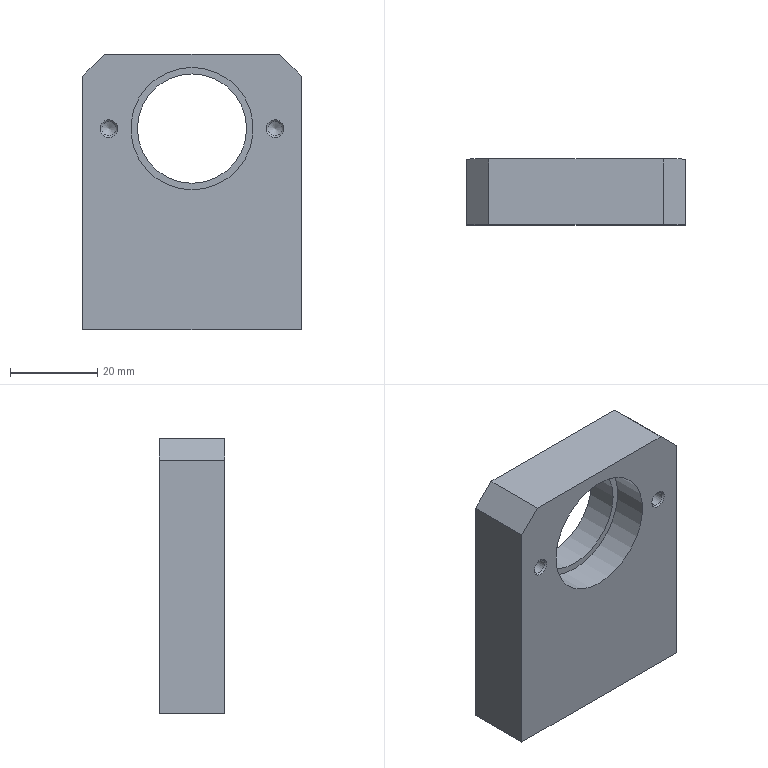Part | NX | 1 solid | 23 faces | box 50 x 15 x 63 mm | volume 38157 mm3 | plane 9 | cone 8 | cylinder 6 | commonest cylinder face diameters 3.3 x4 25 x1 28 x1
STEP:
#1=CARTESIAN_POINT('',(10739.61,-3350.549,-434.902));
#2=VERTEX_POINT('',#1);
#3=CARTESIAN_POINT('',(10739.61,-3350.549,-492.902));
#4=VERTEX_POINT('',#3);
#5=CARTESIAN_POINT('',(10739.61,-3350.549,-434.902));
#6=DIRECTION('',(0.,0.,-1.));
#7=VECTOR('',#6,1.);
#8=LINE('',#5,#7);
#9=EDGE_CURVE('',#2,#4,#8,.T.);
#10=ORIENTED_EDGE('',*,*,#9,.T.);
#11=CARTESIAN_POINT('',(10739.61,-3365.549,-492.902));
#12=VERTEX_POINT('',#11);
#13=CARTESIAN_POINT('',(10739.61,-3365.549,-492.902));
#14=DIRECTION('',(0.,1.,0.));
#15=VECTOR('',#14,1.);
#16=LINE('',#13,#15);
#17=EDGE_CURVE('',#12,#4,#16,.T.);
#18=ORIENTED_EDGE('',*,*,#17,.F.);
#19=CARTESIAN_POINT('',(10739.61,-3365.549,-434.902));
#20=VERTEX_POINT('',#19);
#21=CARTESIAN_POINT('',(10739.61,-3365.549,-434.902));
#22=DIRECTION('',(0.,0.,-1.));
#23=VECTOR('',#22,1.);
#24=LINE('',#21,#23);
#25=EDGE_CURVE('',#20,#12,#24,.T.);
#26=ORIENTED_EDGE('',*,*,#25,.F.);
#27=CARTESIAN_POINT('',(10739.61,-3365.549,-434.902));
#28=DIRECTION('',(0.,1.,0.));
#29=VECTOR('',#28,1.);
#30=LINE('',#27,#29);
#31=EDGE_CURVE('',#20,#2,#30,.T.);
#32=ORIENTED_EDGE('',*,*,#31,.T.);
#33=EDGE_LOOP('',(#10,#18,#26,#32));
#34=FACE_OUTER_BOUND('',#33,.T.);
#35=CARTESIAN_POINT('',(10739.61,-3365.549,-434.902));
#36=DIRECTION('',(1.,0.,0.));
#37=DIRECTION('',(0.,0.,1.));
#38=AXIS2_PLACEMENT_3D('',#35,#36,#37);
#39=PLANE('',#38);
#40=ADVANCED_FACE('',(#34),#39,.F.);
#41=CARTESIAN_POINT('',(10781.61,-3358.049,-492.902));
#42=VERTEX_POINT('',#41);
#43=CARTESIAN_POINT('',(10779.61,-3358.049,-492.902));
#44=DIRECTION('',(0.,0.,1.));
#45=DIRECTION('',(1.,0.,0.));
#46=AXIS2_PLACEMENT_3D('',#43,#44,#45);
#47=CIRCLE('',#46,2.);
#48=EDGE_CURVE('',#42,#42,#47,.T.);
#49=ORIENTED_EDGE('',*,*,#48,.T.);
#50=EDGE_LOOP('',(#49));
#51=FACE_BOUND('',#50,.T.);
#52=CARTESIAN_POINT('',(10751.61,-3358.049,-492.902));
#53=VERTEX_POINT('',#52);
#54=CARTESIAN_POINT('',(10749.61,-3358.049,-492.902));
#55=DIRECTION('',(0.,0.,1.));
#56=DIRECTION('',(1.,0.,0.));
#57=AXIS2_PLACEMENT_3D('',#54,#55,#56);
#58=CIRCLE('',#57,2.);
#59=EDGE_CURVE('',#53,#53,#58,.T.);
#60=ORIENTED_EDGE('',*,*,#59,.T.);
#61=EDGE_LOOP('',(#60));
#62=FACE_BOUND('',#61,.T.);
#63=CARTESIAN_POINT('',(10789.61,-3350.549,-492.902));
#64=VERTEX_POINT('',#63);
#65=CARTESIAN_POINT('',(10739.61,-3350.549,-492.902));
#66=DIRECTION('',(1.,0.,0.));
#67=VECTOR('',#66,1.);
#68=LINE('',#65,#67);
#69=EDGE_CURVE('',#4,#64,#68,.T.);
#70=ORIENTED_EDGE('',*,*,#69,.T.);
#71=CARTESIAN_POINT('',(10789.61,-3365.549,-492.902));
#72=VERTEX_POINT('',#71);
#73=CARTESIAN_POINT('',(10789.61,-3365.549,-492.902));
#74=DIRECTION('',(0.,1.,0.));
#75=VECTOR('',#74,1.);
#76=LINE('',#73,#75);
#77=EDGE_CURVE('',#72,#64,#76,.T.);
#78=ORIENTED_EDGE('',*,*,#77,.F.);
#79=CARTESIAN_POINT('',(10739.61,-3365.549,-492.902));
#80=DIRECTION('',(1.,0.,0.));
#81=VECTOR('',#80,1.);
#82=LINE('',#79,#81);
#83=EDGE_CURVE('',#12,#72,#82,.T.);
#84=ORIENTED_EDGE('',*,*,#83,.F.);
#85=ORIENTED_EDGE('',*,*,#17,.T.);
#86=EDGE_LOOP('',(#70,#78,#84,#85));
#87=FACE_BOUND('',#86,.T.);
#88=CARTESIAN_POINT('',(10739.61,-3365.549,-492.902));
#89=DIRECTION('',(0.,0.,1.));
#90=DIRECTION('',(-1.,0.,0.));
#91=AXIS2_PLACEMENT_3D('',#88,#89,#90);
#92=PLANE('',#91);
#93=ADVANCED_FACE('',(#51,#62,#87),#92,.F.);
#94=CARTESIAN_POINT('',(10789.61,-3350.549,-434.902));
#95=VERTEX_POINT('',#94);
#96=CARTESIAN_POINT('',(10789.61,-3350.549,-492.902));
#97=DIRECTION('',(0.,0.,1.));
#98=VECTOR('',#97,1.);
#99=LINE('',#96,#98);
#100=EDGE_CURVE('',#64,#95,#99,.T.);
#101=ORIENTED_EDGE('',*,*,#100,.T.);
#102=CARTESIAN_POINT('',(10789.61,-3365.549,-434.902));
#103=VERTEX_POINT('',#102);
#104=CARTESIAN_POINT('',(10789.61,-3365.549,-434.902));
#105=DIRECTION('',(0.,1.,0.));
#106=VECTOR('',#105,1.);
#107=LINE('',#104,#106);
#108=EDGE_CURVE('',#103,#95,#107,.T.);
#109=ORIENTED_EDGE('',*,*,#108,.F.);
#110=CARTESIAN_POINT('',(10789.61,-3365.549,-492.902));
#111=DIRECTION('',(0.,0.,1.));
#112=VECTOR('',#111,1.);
#113=LINE('',#110,#112);
#114=EDGE_CURVE('',#72,#103,#113,.T.);
#115=ORIENTED_EDGE('',*,*,#114,.F.);
#116=ORIENTED_EDGE('',*,*,#77,.T.);
#117=EDGE_LOOP('',(#101,#109,#115,#116));
#118=FACE_OUTER_BOUND('',#117,.T.);
#119=CARTESIAN_POINT('',(10789.61,-3365.549,-492.902));
#120=DIRECTION('',(-1.,0.,0.));
#121=DIRECTION('',(0.,0.,-1.));
#122=AXIS2_PLACEMENT_3D('',#119,#120,#121);
#123=PLANE('',#122);
#124=ADVANCED_FACE('',(#118),#123,.F.);
#125=CARTESIAN_POINT('',(10784.61,-3350.549,-429.902));
#126=VERTEX_POINT('',#125);
#127=CARTESIAN_POINT('',(10789.61,-3350.549,-434.902));
#128=DIRECTION('',(-0.7071,0.,0.7071));
#129=VECTOR('',#128,1.);
#130=LINE('',#127,#129);
#131=EDGE_CURVE('',#95,#126,#130,.T.);
#132=ORIENTED_EDGE('',*,*,#131,.T.);
#133=CARTESIAN_POINT('',(10784.61,-3365.549,-429.902));
#134=VERTEX_POINT('',#133);
#135=CARTESIAN_POINT('',(10784.61,-3365.549,-429.902));
#136=DIRECTION('',(0.,1.,0.));
#137=VECTOR('',#136,1.);
#138=LINE('',#135,#137);
#139=EDGE_CURVE('',#134,#126,#138,.T.);
#140=ORIENTED_EDGE('',*,*,#139,.F.);
#141=CARTESIAN_POINT('',(10789.61,-3365.549,-434.902));
#142=DIRECTION('',(-0.7071,0.,0.7071));
#143=VECTOR('',#142,1.);
#144=LINE('',#141,#143);
#145=EDGE_CURVE('',#103,#134,#144,.T.);
#146=ORIENTED_EDGE('',*,*,#145,.F.);
#147=ORIENTED_EDGE('',*,*,#108,.T.);
#148=EDGE_LOOP('',(#132,#140,#146,#147));
#149=FACE_OUTER_BOUND('',#148,.T.);
#150=CARTESIAN_POINT('',(10789.61,-3365.549,-434.902));
#151=DIRECTION('',(-0.7071,0.,-0.7071));
#152=DIRECTION('',(0.7071,0.,-0.7071));
#153=AXIS2_PLACEMENT_3D('',#150,#151,#152);
#154=PLANE('',#153);
#155=ADVANCED_FACE('',(#149),#154,.F.);
#156=CARTESIAN_POINT('',(10744.61,-3350.549,-429.902));
#157=VERTEX_POINT('',#156);
#158=CARTESIAN_POINT('',(10784.61,-3350.549,-429.902));
#159=DIRECTION('',(-1.,0.,0.));
#160=VECTOR('',#159,1.);
#161=LINE('',#158,#160);
#162=EDGE_CURVE('',#126,#157,#161,.T.);
#163=ORIENTED_EDGE('',*,*,#162,.T.);
#164=CARTESIAN_POINT('',(10744.61,-3365.549,-429.902));
#165=VERTEX_POINT('',#164);
#166=CARTESIAN_POINT('',(10744.61,-3365.549,-429.902));
#167=DIRECTION('',(0.,1.,0.));
#168=VECTOR('',#167,1.);
#169=LINE('',#166,#168);
#170=EDGE_CURVE('',#165,#157,#169,.T.);
#171=ORIENTED_EDGE('',*,*,#170,.F.);
#172=CARTESIAN_POINT('',(10784.61,-3365.549,-429.902));
#173=DIRECTION('',(-1.,0.,0.));
#174=VECTOR('',#173,1.);
#175=LINE('',#172,#174);
#176=EDGE_CURVE('',#134,#165,#175,.T.);
#177=ORIENTED_EDGE('',*,*,#176,.F.);
#178=ORIENTED_EDGE('',*,*,#139,.T.);
#179=EDGE_LOOP('',(#163,#171,#177,#178));
#180=FACE_OUTER_BOUND('',#179,.T.);
#181=CARTESIAN_POINT('',(10784.61,-3365.549,-429.902));
#182=DIRECTION('',(0.,0.,-1.));
#183=DIRECTION('',(1.,0.,0.));
#184=AXIS2_PLACEMENT_3D('',#181,#182,#183);
#185=PLANE('',#184);
#186=ADVANCED_FACE('',(#180),#185,.F.);
#187=CARTESIAN_POINT('',(10744.61,-3350.549,-429.902));
#188=DIRECTION('',(-0.7071,0.,-0.7071));
#189=VECTOR('',#188,1.);
#190=LINE('',#187,#189);
#191=EDGE_CURVE('',#157,#2,#190,.T.);
#192=ORIENTED_EDGE('',*,*,#191,.T.);
#193=ORIENTED_EDGE('',*,*,#31,.F.);
#194=CARTESIAN_POINT('',(10744.61,-3365.549,-429.902));
#195=DIRECTION('',(-0.7071,0.,-0.7071));
#196=VECTOR('',#195,1.);
#197=LINE('',#194,#196);
#198=EDGE_CURVE('',#165,#20,#197,.T.);
#199=ORIENTED_EDGE('',*,*,#198,.F.);
#200=ORIENTED_EDGE('',*,*,#170,.T.);
#201=EDGE_LOOP('',(#192,#193,#199,#200));
#202=FACE_OUTER_BOUND('',#201,.T.);
#203=CARTESIAN_POINT('',(10744.61,-3365.549,-429.902));
#204=DIRECTION('',(0.7071,0.,-0.7071));
#205=DIRECTION('',(0.7071,0.,0.7071));
#206=AXIS2_PLACEMENT_3D('',#203,#204,#205);
#207=PLANE('',#206);
#208=ADVANCED_FACE('',(#202),#207,.F.);
#209=CARTESIAN_POINT('',(10764.61,-3357.549,-434.402));
#210=VERTEX_POINT('',#209);
#211=CARTESIAN_POINT('',(10764.61,-3357.549,-446.902));
#212=DIRECTION('',(0.,1.,0.));
#213=DIRECTION('',(0.,0.,1.));
#214=AXIS2_PLACEMENT_3D('',#211,#212,#213);
#215=CIRCLE('',#214,12.5);
#216=EDGE_CURVE('',#210,#210,#215,.T.);
#217=ORIENTED_EDGE('',*,*,#216,.F.);
#218=EDGE_LOOP('',(#217));
#219=FACE_BOUND('',#218,.T.);
#220=CARTESIAN_POINT('',(10764.61,-3350.549,-459.402));
#221=VERTEX_POINT('',#220);
#222=CARTESIAN_POINT('',(10764.61,-3350.549,-446.902));
#223=DIRECTION('',(0.,-1.,0.));
#224=DIRECTION('',(0.,0.,-1.));
#225=AXIS2_PLACEMENT_3D('',#222,#223,#224);
#226=CIRCLE('',#225,12.5);
#227=EDGE_CURVE('',#221,#221,#226,.T.);
#228=ORIENTED_EDGE('',*,*,#227,.F.);
#229=EDGE_LOOP('',(#228));
#230=FACE_BOUND('',#229,.T.);
#231=CARTESIAN_POINT('',(10764.61,-3365.549,-446.902));
#232=DIRECTION('',(0.,1.,0.));
#233=DIRECTION('',(0.,0.,-1.));
#234=AXIS2_PLACEMENT_3D('',#231,#232,#233);
#235=CYLINDRICAL_SURFACE('',#234,12.5);
#236=ADVANCED_FACE('',(#219,#230),#235,.F.);
#237=CARTESIAN_POINT('',(10783.61,-3365.549,-448.902));
#238=VERTEX_POINT('',#237);
#239=CARTESIAN_POINT('',(10783.61,-3365.549,-446.902));
#240=DIRECTION('',(0.,1.,0.));
#241=DIRECTION('',(0.,0.,-1.));
#242=AXIS2_PLACEMENT_3D('',#239,#240,#241);
#243=CIRCLE('',#242,2.);
#244=EDGE_CURVE('',#238,#238,#243,.T.);
#245=ORIENTED_EDGE('',*,*,#244,.T.);
#246=EDGE_LOOP('',(#245));
#247=FACE_BOUND('',#246,.T.);
#248=CARTESIAN_POINT('',(10745.61,-3365.549,-448.902));
#249=VERTEX_POINT('',#248);
#250=CARTESIAN_POINT('',(10745.61,-3365.549,-446.902));
#251=DIRECTION('',(0.,1.,0.));
#252=DIRECTION('',(0.,0.,-1.));
#253=AXIS2_PLACEMENT_3D('',#250,#251,#252);
#254=CIRCLE('',#253,2.);
#255=EDGE_CURVE('',#249,#249,#254,.T.);
#256=ORIENTED_EDGE('',*,*,#255,.T.);
#257=EDGE_LOOP('',(#256));
#258=FACE_BOUND('',#257,.T.);
#259=CARTESIAN_POINT('',(10764.61,-3365.549,-460.902));
#260=VERTEX_POINT('',#259);
#261=CARTESIAN_POINT('',(10764.61,-3365.549,-446.902));
#262=DIRECTION('',(0.,1.,0.));
#263=DIRECTION('',(0.,0.,-1.));
#264=AXIS2_PLACEMENT_3D('',#261,#262,#263);
#265=CIRCLE('',#264,14.);
#266=EDGE_CURVE('',#260,#260,#265,.T.);
#267=ORIENTED_EDGE('',*,*,#266,.T.);
#268=EDGE_LOOP('',(#267));
#269=FACE_BOUND('',#268,.T.);
#270=ORIENTED_EDGE('',*,*,#25,.T.);
#271=ORIENTED_EDGE('',*,*,#83,.T.);
#272=ORIENTED_EDGE('',*,*,#114,.T.);
#273=ORIENTED_EDGE('',*,*,#145,.T.);
#274=ORIENTED_EDGE('',*,*,#176,.T.);
#275=ORIENTED_EDGE('',*,*,#198,.T.);
#276=EDGE_LOOP('',(#270,#271,#272,#273,#274,#275));
#277=FACE_BOUND('',#276,.T.);
#278=CARTESIAN_POINT('',(10764.61,-3365.549,-446.902));
#279=DIRECTION('',(0.,-1.,0.));
#280=DIRECTION('',(0.,0.,1.));
#281=AXIS2_PLACEMENT_3D('',#278,#279,#280);
#282=PLANE('',#281);
#283=ADVANCED_FACE('',(#247,#258,#269,#277),#282,.T.);
#284=ORIENTED_EDGE('',*,*,#9,.F.);
#285=ORIENTED_EDGE('',*,*,#191,.F.);
#286=ORIENTED_EDGE('',*,*,#162,.F.);
#287=ORIENTED_EDGE('',*,*,#131,.F.);
#288=ORIENTED_EDGE('',*,*,#100,.F.);
#289=ORIENTED_EDGE('',*,*,#69,.F.);
#290=EDGE_LOOP('',(#284,#285,#286,#287,#288,#289));
#291=FACE_BOUND('',#290,.T.);
#292=ORIENTED_EDGE('',*,*,#227,.T.);
#293=EDGE_LOOP('',(#292));
#294=FACE_BOUND('',#293,.T.);
#295=CARTESIAN_POINT('',(10764.61,-3350.549,-446.902));
#296=DIRECTION('',(0.,-1.,0.));
#297=DIRECTION('',(0.,0.,1.));
#298=AXIS2_PLACEMENT_3D('',#295,#296,#297);
#299=PLANE('',#298);
#300=ADVANCED_FACE('',(#291,#294),#299,.F.);
#301=CARTESIAN_POINT('',(10764.61,-3357.549,-460.902));
#302=VERTEX_POINT('',#301);
#303=CARTESIAN_POINT('',(10764.61,-3357.549,-446.902));
#304=DIRECTION('',(0.,-1.,0.));
#305=DIRECTION('',(0.,0.,-1.));
#306=AXIS2_PLACEMENT_3D('',#303,#304,#305);
#307=CIRCLE('',#306,14.);
#308=EDGE_CURVE('',#302,#302,#307,.T.);
#309=ORIENTED_EDGE('',*,*,#308,.F.);
#310=EDGE_LOOP('',(#309));
#311=FACE_BOUND('',#310,.T.);
#312=ORIENTED_EDGE('',*,*,#266,.F.);
#313=EDGE_LOOP('',(#312));
#314=FACE_BOUND('',#313,.T.);
#315=CARTESIAN_POINT('',(10764.61,-3365.549,-446.902));
#316=DIRECTION('',(0.,1.,0.));
#317=DIRECTION('',(0.,0.,-1.));
#318=AXIS2_PLACEMENT_3D('',#315,#316,#317);
#319=CYLINDRICAL_SURFACE('',#318,14.);
#320=ADVANCED_FACE('',(#311,#314),#319,.F.);
#321=ORIENTED_EDGE('',*,*,#216,.T.);
#322=EDGE_LOOP('',(#321));
#323=FACE_BOUND('',#322,.T.);
#324=ORIENTED_EDGE('',*,*,#308,.T.);
#325=EDGE_LOOP('',(#324));
#326=FACE_BOUND('',#325,.T.);
#327=CARTESIAN_POINT('',(10764.61,-3357.549,-446.902));
#328=DIRECTION('',(0.,1.,0.));
#329=DIRECTION('',(0.,0.,-1.));
#330=AXIS2_PLACEMENT_3D('',#327,#328,#329);
#331=PLANE('',#330);
#332=ADVANCED_FACE('',(#323,#326),#331,.F.);
#333=CARTESIAN_POINT('',(10745.61,-3355.549,-445.252));
#334=VERTEX_POINT('',#333);
#335=CARTESIAN_POINT('',(10745.61,-3355.549,-446.902));
#336=DIRECTION('',(0.,-1.,0.));
#337=DIRECTION('',(0.,0.,1.));
#338=AXIS2_PLACEMENT_3D('',#335,#336,#337);
#339=CIRCLE('',#338,1.65);
#340=EDGE_CURVE('',#334,#334,#339,.T.);
#341=ORIENTED_EDGE('',*,*,#340,.T.);
#342=EDGE_LOOP('',(#341));
#343=FACE_BOUND('',#342,.T.);
#344=CARTESIAN_POINT('',(10745.61,-3354.558,-446.902));
#345=VERTEX_POINT('',#344);
#346=VERTEX_LOOP('',#345);
#347=FACE_BOUND('',#346,.T.);
#348=CARTESIAN_POINT('',(10745.61,-3355.549,-446.902));
#349=DIRECTION('',(0.,-1.,0.));
#350=DIRECTION('',(0.,0.,1.));
#351=AXIS2_PLACEMENT_3D('',#348,#349,#350);
#352=CONICAL_SURFACE('',#351,1.65,59.);
#353=ADVANCED_FACE('',(#343,#347),#352,.F.);
#354=CARTESIAN_POINT('',(10745.61,-3365.199,-448.552));
#355=VERTEX_POINT('',#354);
#356=CARTESIAN_POINT('',(10745.61,-3365.199,-446.902));
#357=DIRECTION('',(0.,-1.,0.));
#358=DIRECTION('',(0.,0.,-1.));
#359=AXIS2_PLACEMENT_3D('',#356,#357,#358);
#360=CIRCLE('',#359,1.65);
#361=EDGE_CURVE('',#355,#355,#360,.T.);
#362=ORIENTED_EDGE('',*,*,#361,.T.);
#363=EDGE_LOOP('',(#362));
#364=FACE_BOUND('',#363,.T.);
#365=ORIENTED_EDGE('',*,*,#340,.F.);
#366=EDGE_LOOP('',(#365));
#367=FACE_BOUND('',#366,.T.);
#368=CARTESIAN_POINT('',(10745.61,-3365.549,-446.902));
#369=DIRECTION('',(0.,1.,0.));
#370=DIRECTION('',(0.,0.,-1.));
#371=AXIS2_PLACEMENT_3D('',#368,#369,#370);
#372=CYLINDRICAL_SURFACE('',#371,1.65);
#373=ADVANCED_FACE('',(#364,#367),#372,.F.);
#374=ORIENTED_EDGE('',*,*,#361,.F.);
#375=EDGE_LOOP('',(#374));
#376=FACE_BOUND('',#375,.T.);
#377=ORIENTED_EDGE('',*,*,#255,.F.);
#378=EDGE_LOOP('',(#377));
#379=FACE_BOUND('',#378,.T.);
#380=CARTESIAN_POINT('',(10745.61,-3365.549,-446.902));
#381=DIRECTION('',(0.,-1.,0.));
#382=DIRECTION('',(0.,0.,1.));
#383=AXIS2_PLACEMENT_3D('',#380,#381,#382);
#384=CONICAL_SURFACE('',#383,2.,45.);
#385=ADVANCED_FACE('',(#376,#379),#384,.F.);
#386=CARTESIAN_POINT('',(10751.26,-3358.049,-482.902));
#387=VERTEX_POINT('',#386);
#388=CARTESIAN_POINT('',(10749.61,-3358.049,-482.902));
#389=DIRECTION('',(0.,0.,-1.));
#390=DIRECTION('',(1.,0.,0.));
#391=AXIS2_PLACEMENT_3D('',#388,#389,#390);
#392=CIRCLE('',#391,1.65);
#393=EDGE_CURVE('',#387,#387,#392,.T.);
#394=ORIENTED_EDGE('',*,*,#393,.T.);
#395=EDGE_LOOP('',(#394));
#396=FACE_BOUND('',#395,.T.);
#397=CARTESIAN_POINT('',(10749.61,-3358.049,-481.911));
#398=VERTEX_POINT('',#397);
#399=VERTEX_LOOP('',#398);
#400=FACE_BOUND('',#399,.T.);
#401=CARTESIAN_POINT('',(10749.61,-3358.049,-482.902));
#402=DIRECTION('',(0.,0.,-1.));
#403=DIRECTION('',(1.,0.,0.));
#404=AXIS2_PLACEMENT_3D('',#401,#402,#403);
#405=CONICAL_SURFACE('',#404,1.65,59.);
#406=ADVANCED_FACE('',(#396,#400),#405,.F.);
#407=CARTESIAN_POINT('',(10751.26,-3358.049,-492.552));
#408=VERTEX_POINT('',#407);
#409=CARTESIAN_POINT('',(10749.61,-3358.049,-492.552));
#410=DIRECTION('',(0.,0.,-1.));
#411=DIRECTION('',(1.,0.,0.));
#412=AXIS2_PLACEMENT_3D('',#409,#410,#411);
#413=CIRCLE('',#412,1.65);
#414=EDGE_CURVE('',#408,#408,#413,.T.);
#415=ORIENTED_EDGE('',*,*,#414,.T.);
#416=EDGE_LOOP('',(#415));
#417=FACE_BOUND('',#416,.T.);
#418=ORIENTED_EDGE('',*,*,#393,.F.);
#419=EDGE_LOOP('',(#418));
#420=FACE_BOUND('',#419,.T.);
#421=CARTESIAN_POINT('',(10749.61,-3358.049,-492.902));
#422=DIRECTION('',(0.,0.,1.));
#423=DIRECTION('',(-1.,0.,0.));
#424=AXIS2_PLACEMENT_3D('',#421,#422,#423);
#425=CYLINDRICAL_SURFACE('',#424,1.65);
#426=ADVANCED_FACE('',(#417,#420),#425,.F.);
#427=ORIENTED_EDGE('',*,*,#414,.F.);
#428=EDGE_LOOP('',(#427));
#429=FACE_BOUND('',#428,.T.);
#430=ORIENTED_EDGE('',*,*,#59,.F.);
#431=EDGE_LOOP('',(#430));
#432=FACE_BOUND('',#431,.T.);
#433=CARTESIAN_POINT('',(10749.61,-3358.049,-492.902));
#434=DIRECTION('',(0.,0.,-1.));
#435=DIRECTION('',(1.,0.,0.));
#436=AXIS2_PLACEMENT_3D('',#433,#434,#435);
#437=CONICAL_SURFACE('',#436,2.,45.);
#438=ADVANCED_FACE('',(#429,#432),#437,.F.);
#439=CARTESIAN_POINT('',(10783.61,-3355.549,-445.252));
#440=VERTEX_POINT('',#439);
#441=CARTESIAN_POINT('',(10783.61,-3355.549,-446.902));
#442=DIRECTION('',(0.,1.,0.));
#443=DIRECTION('',(0.,0.,1.));
#444=AXIS2_PLACEMENT_3D('',#441,#442,#443);
#445=CIRCLE('',#444,1.65);
#446=EDGE_CURVE('',#440,#440,#445,.T.);
#447=ORIENTED_EDGE('',*,*,#446,.F.);
#448=EDGE_LOOP('',(#447));
#449=FACE_BOUND('',#448,.T.);
#450=CARTESIAN_POINT('',(10783.61,-3354.558,-446.902));
#451=VERTEX_POINT('',#450);
#452=VERTEX_LOOP('',#451);
#453=FACE_BOUND('',#452,.T.);
#454=CARTESIAN_POINT('',(10783.61,-3355.549,-446.902));
#455=DIRECTION('',(0.,-1.,0.));
#456=DIRECTION('',(0.,0.,1.));
#457=AXIS2_PLACEMENT_3D('',#454,#455,#456);
#458=CONICAL_SURFACE('',#457,1.65,59.);
#459=ADVANCED_FACE('',(#449,#453),#458,.F.);
#460=CARTESIAN_POINT('',(10783.61,-3365.199,-448.552));
#461=VERTEX_POINT('',#460);
#462=CARTESIAN_POINT('',(10783.61,-3365.199,-446.902));
#463=DIRECTION('',(0.,1.,0.));
#464=DIRECTION('',(0.,0.,-1.));
#465=AXIS2_PLACEMENT_3D('',#462,#463,#464);
#466=CIRCLE('',#465,1.65);
#467=EDGE_CURVE('',#461,#461,#466,.T.);
#468=ORIENTED_EDGE('',*,*,#467,.F.);
#469=EDGE_LOOP('',(#468));
#470=FACE_BOUND('',#469,.T.);
#471=ORIENTED_EDGE('',*,*,#446,.T.);
#472=EDGE_LOOP('',(#471));
#473=FACE_BOUND('',#472,.T.);
#474=CARTESIAN_POINT('',(10783.61,-3365.549,-446.902));
#475=DIRECTION('',(0.,1.,0.));
#476=DIRECTION('',(0.,0.,-1.));
#477=AXIS2_PLACEMENT_3D('',#474,#475,#476);
#478=CYLINDRICAL_SURFACE('',#477,1.65);
#479=ADVANCED_FACE('',(#470,#473),#478,.F.);
#480=ORIENTED_EDGE('',*,*,#467,.T.);
#481=EDGE_LOOP('',(#480));
#482=FACE_BOUND('',#481,.T.);
#483=ORIENTED_EDGE('',*,*,#244,.F.);
#484=EDGE_LOOP('',(#483));
#485=FACE_BOUND('',#484,.T.);
#486=CARTESIAN_POINT('',(10783.61,-3365.549,-446.902));
#487=DIRECTION('',(0.,-1.,0.));
#488=DIRECTION('',(0.,0.,1.));
#489=AXIS2_PLACEMENT_3D('',#486,#487,#488);
#490=CONICAL_SURFACE('',#489,2.,45.);
#491=ADVANCED_FACE('',(#482,#485),#490,.F.);
#492=CARTESIAN_POINT('',(10781.26,-3358.049,-482.902));
#493=VERTEX_POINT('',#492);
#494=CARTESIAN_POINT('',(10779.61,-3358.049,-482.902));
#495=DIRECTION('',(0.,0.,1.));
#496=DIRECTION('',(1.,0.,0.));
#497=AXIS2_PLACEMENT_3D('',#494,#495,#496);
#498=CIRCLE('',#497,1.65);
#499=EDGE_CURVE('',#493,#493,#498,.T.);
#500=ORIENTED_EDGE('',*,*,#499,.F.);
#501=EDGE_LOOP('',(#500));
#502=FACE_BOUND('',#501,.T.);
#503=CARTESIAN_POINT('',(10779.61,-3358.049,-481.911));
#504=VERTEX_POINT('',#503);
#505=VERTEX_LOOP('',#504);
#506=FACE_BOUND('',#505,.T.);
#507=CARTESIAN_POINT('',(10779.61,-3358.049,-482.902));
#508=DIRECTION('',(0.,0.,-1.));
#509=DIRECTION('',(1.,0.,0.));
#510=AXIS2_PLACEMENT_3D('',#507,#508,#509);
#511=CONICAL_SURFACE('',#510,1.65,59.);
#512=ADVANCED_FACE('',(#502,#506),#511,.F.);
#513=CARTESIAN_POINT('',(10781.26,-3358.049,-492.552));
#514=VERTEX_POINT('',#513);
#515=CARTESIAN_POINT('',(10779.61,-3358.049,-492.552));
#516=DIRECTION('',(0.,0.,1.));
#517=DIRECTION('',(1.,0.,0.));
#518=AXIS2_PLACEMENT_3D('',#515,#516,#517);
#519=CIRCLE('',#518,1.65);
#520=EDGE_CURVE('',#514,#514,#519,.T.);
#521=ORIENTED_EDGE('',*,*,#520,.F.);
#522=EDGE_LOOP('',(#521));
#523=FACE_BOUND('',#522,.T.);
#524=ORIENTED_EDGE('',*,*,#499,.T.);
#525=EDGE_LOOP('',(#524));
#526=FACE_BOUND('',#525,.T.);
#527=CARTESIAN_POINT('',(10779.61,-3358.049,-492.902));
#528=DIRECTION('',(0.,0.,1.));
#529=DIRECTION('',(-1.,0.,0.));
#530=AXIS2_PLACEMENT_3D('',#527,#528,#529);
#531=CYLINDRICAL_SURFACE('',#530,1.65);
#532=ADVANCED_FACE('',(#523,#526),#531,.F.);
#533=ORIENTED_EDGE('',*,*,#520,.T.);
#534=EDGE_LOOP('',(#533));
#535=FACE_BOUND('',#534,.T.);
#536=ORIENTED_EDGE('',*,*,#48,.F.);
#537=EDGE_LOOP('',(#536));
#538=FACE_BOUND('',#537,.T.);
#539=CARTESIAN_POINT('',(10779.61,-3358.049,-492.902));
#540=DIRECTION('',(0.,0.,-1.));
#541=DIRECTION('',(1.,0.,0.));
#542=AXIS2_PLACEMENT_3D('',#539,#540,#541);
#543=CONICAL_SURFACE('',#542,2.,45.);
#544=ADVANCED_FACE('',(#535,#538),#543,.F.);
#545=CLOSED_SHELL('',(#40,#93,#124,#155,#186,#208,#236,#283,#300,#320,#332,#353,#373,#385,#406,#426,#438,#459,#479,#491,#512,#532,#544));
#546=MANIFOLD_SOLID_BREP('',#545);
#547=(LENGTH_UNIT()NAMED_UNIT(*)SI_UNIT(.MILLI.,.METRE.));
#548=UNCERTAINTY_MEASURE_WITH_UNIT(LENGTH_MEASURE(0.00002),#547,'','');
#549=(NAMED_UNIT(*)PLANE_ANGLE_UNIT()SI_UNIT($,.RADIAN.));
#550=PLANE_ANGLE_MEASURE_WITH_UNIT(PLANE_ANGLE_MEASURE(0.01745),#549);
#551=DIMENSIONAL_EXPONENTS(0.,0.,0.,0.,0.,0.,0.);
#552=(CONVERSION_BASED_UNIT('DEGREE',#550)NAMED_UNIT(#551)PLANE_ANGLE_UNIT());
#553=(NAMED_UNIT(*)SI_UNIT($,.STERADIAN.)SOLID_ANGLE_UNIT());
#554=(GEOMETRIC_REPRESENTATION_CONTEXT(3)GLOBAL_UNCERTAINTY_ASSIGNED_CONTEXT((#548))GLOBAL_UNIT_ASSIGNED_CONTEXT((#547,#552,#553))REPRESENTATION_CONTEXT('',''));
#555=ADVANCED_BREP_SHAPE_REPRESENTATION('',(#546),#554);